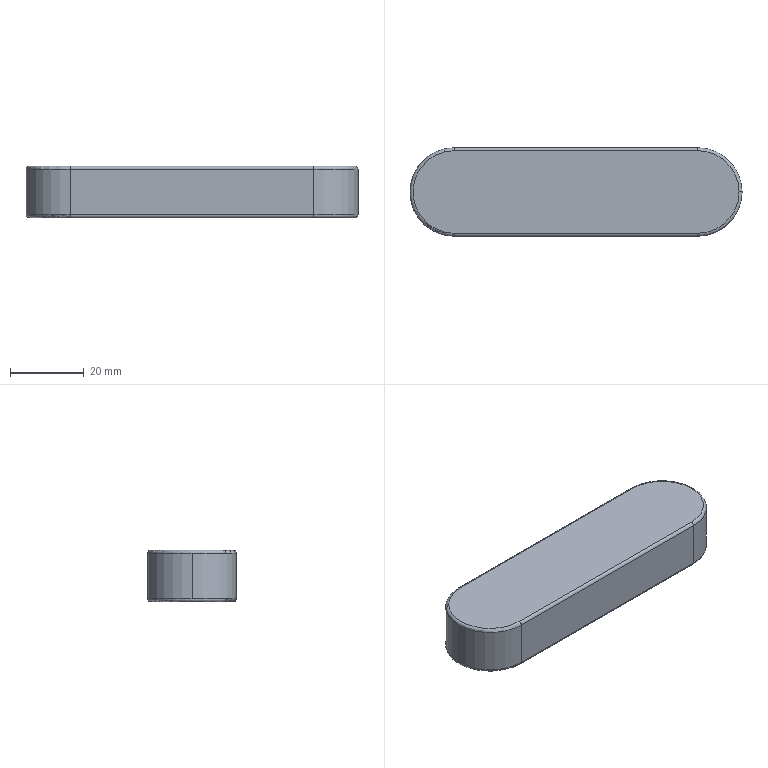Part | STEP file | GB/T1096-1979 plain key, type A, 24×90 | 1 solid | 17 faces | box 90 x 24 x 14 mm | volume 28453 mm3 | cylinder 7 | torus 6 | plane 4 | commonest cylinder face diameters 1.6 x4 24 x3
STEP:
#1=CARTESIAN_POINT('',(0.,0.,0.));
#2=DIRECTION('',(0.,0.,1.));
#3=DIRECTION('',(1.,0.,0.));
#4=AXIS2_PLACEMENT_3D('',#1,#2,#3);
#5=CARTESIAN_POINT('',(44.2,0.,0.));
#6=VERTEX_POINT('',#5);
#7=CARTESIAN_POINT('',(33.,-11.2,0.));
#8=VERTEX_POINT('',#7);
#9=CARTESIAN_POINT('',(33.,0.,0.));
#10=DIRECTION('',(0.,0.,-1.));
#11=DIRECTION('',(1.,0.,0.));
#12=AXIS2_PLACEMENT_3D('',#9,#10,#11);
#13=CIRCLE('',#12,11.2);
#14=CARTESIAN_POINT('',(33.,0.,0.8));
#15=DIRECTION('',(0.,0.,1.));
#16=DIRECTION('',(1.,0.,0.));
#17=AXIS2_PLACEMENT_3D('',#14,#15,#16);
#18=TOROIDAL_SURFACE('',#17,11.2,0.8);
#19=CARTESIAN_POINT('',(6.283,4.712));
#20=DIRECTION('',(-1.,0.));
#21=VECTOR('',#20,1.);
#22=LINE('',#19,#21);
#23=(GEOMETRIC_REPRESENTATION_CONTEXT(2)PARAMETRIC_REPRESENTATION_CONTEXT()REPRESENTATION_CONTEXT('',''));
#24=DEFINITIONAL_REPRESENTATION('',(#22),#23);
#25=PCURVE('',#18,#24);
#26=CARTESIAN_POINT('',(-33.,0.,0.));
#27=DIRECTION('',(0.,0.,1.));
#28=DIRECTION('',(1.,0.,0.));
#29=AXIS2_PLACEMENT_3D('',#26,#27,#28);
#30=PLANE('',#29);
#31=CARTESIAN_POINT('',(77.2,0.));
#32=CARTESIAN_POINT('',(77.2,-19.399));
#33=CARTESIAN_POINT('',(60.4,-9.699));
#34=CARTESIAN_POINT('',(43.6,0.));
#35=CARTESIAN_POINT('',(60.4,9.699));
#36=CARTESIAN_POINT('',(77.2,19.399));
#37=CARTESIAN_POINT('',(77.2,0.));
#38=(BOUNDED_CURVE()B_SPLINE_CURVE(2,(#31,#32,#33,#34,#35,#36,#37),.UNSPECIFIED.,.T.,.F.)B_SPLINE_CURVE_WITH_KNOTS((1,2,2,2,2,1),(-2.094,0.,2.094,4.189,6.283,8.378),.UNSPECIFIED.)CURVE()GEOMETRIC_REPRESENTATION_ITEM()RATIONAL_B_SPLINE_CURVE((1.,0.5,1.,0.5,1.,0.5,1.))REPRESENTATION_ITEM(''));
#39=(GEOMETRIC_REPRESENTATION_CONTEXT(2)PARAMETRIC_REPRESENTATION_CONTEXT()REPRESENTATION_CONTEXT('',''));
#40=DEFINITIONAL_REPRESENTATION('',(#38),#39);
#41=PCURVE('',#30,#40);
#42=SURFACE_CURVE('',#13,(#25,#41),.PCURVE_S1.);
#43=EDGE_CURVE('',#6,#8,#42,.T.);
#44=ORIENTED_EDGE('',*,*,#43,.F.);
#45=CARTESIAN_POINT('',(45.,0.,0.8));
#46=VERTEX_POINT('',#45);
#47=CARTESIAN_POINT('',(44.2,0.,0.8));
#48=DIRECTION('',(0.,-1.,0.));
#49=DIRECTION('',(0.,0.,-1.));
#50=AXIS2_PLACEMENT_3D('',#47,#48,#49);
#51=CIRCLE('',#50,0.8);
#52=CARTESIAN_POINT('',(6.283,4.712));
#53=DIRECTION('',(0.,1.));
#54=VECTOR('',#53,1.);
#55=LINE('',#52,#54);
#56=(GEOMETRIC_REPRESENTATION_CONTEXT(2)PARAMETRIC_REPRESENTATION_CONTEXT()REPRESENTATION_CONTEXT('',''));
#57=DEFINITIONAL_REPRESENTATION('',(#55),#56);
#58=PCURVE('',#18,#57);
#59=CARTESIAN_POINT('',(33.,0.,0.8));
#60=DIRECTION('',(0.,0.,1.));
#61=DIRECTION('',(1.,0.,0.));
#62=AXIS2_PLACEMENT_3D('',#59,#60,#61);
#63=TOROIDAL_SURFACE('',#62,11.2,0.8);
#64=CARTESIAN_POINT('',(0.,4.712));
#65=DIRECTION('',(0.,1.));
#66=VECTOR('',#65,1.);
#67=LINE('',#64,#66);
#68=(GEOMETRIC_REPRESENTATION_CONTEXT(2)PARAMETRIC_REPRESENTATION_CONTEXT()REPRESENTATION_CONTEXT('',''));
#69=DEFINITIONAL_REPRESENTATION('',(#67),#68);
#70=PCURVE('',#63,#69);
#71=SURFACE_CURVE('',#51,(#58,#70),.PCURVE_S1.);
#72=EDGE_CURVE('',#6,#46,#71,.T.);
#73=ORIENTED_EDGE('',*,*,#72,.T.);
#74=CARTESIAN_POINT('',(33.,-12.,0.8));
#75=VERTEX_POINT('',#74);
#76=CARTESIAN_POINT('',(33.,0.,0.8));
#77=DIRECTION('',(0.,0.,1.));
#78=DIRECTION('',(1.,0.,0.));
#79=AXIS2_PLACEMENT_3D('',#76,#77,#78);
#80=CIRCLE('',#79,12.);
#81=CARTESIAN_POINT('',(0.,6.283));
#82=DIRECTION('',(1.,0.));
#83=VECTOR('',#82,1.);
#84=LINE('',#81,#83);
#85=(GEOMETRIC_REPRESENTATION_CONTEXT(2)PARAMETRIC_REPRESENTATION_CONTEXT()REPRESENTATION_CONTEXT('',''));
#86=DEFINITIONAL_REPRESENTATION('',(#84),#85);
#87=PCURVE('',#18,#86);
#88=CARTESIAN_POINT('',(33.,0.,14.));
#89=DIRECTION('',(0.,0.,-1.));
#90=DIRECTION('',(-1.,0.,0.));
#91=AXIS2_PLACEMENT_3D('',#88,#89,#90);
#92=CYLINDRICAL_SURFACE('',#91,12.);
#93=CARTESIAN_POINT('',(9.425,13.2));
#94=DIRECTION('',(-1.,0.));
#95=VECTOR('',#94,1.);
#96=LINE('',#93,#95);
#97=(GEOMETRIC_REPRESENTATION_CONTEXT(2)PARAMETRIC_REPRESENTATION_CONTEXT()REPRESENTATION_CONTEXT('',''));
#98=DEFINITIONAL_REPRESENTATION('',(#96),#97);
#99=PCURVE('',#92,#98);
#100=SURFACE_CURVE('',#80,(#87,#99),.PCURVE_S1.);
#101=EDGE_CURVE('',#75,#46,#100,.T.);
#102=ORIENTED_EDGE('',*,*,#101,.F.);
#103=CARTESIAN_POINT('',(33.,-11.2,0.8));
#104=DIRECTION('',(1.,0.,0.));
#105=DIRECTION('',(0.,0.,-1.));
#106=AXIS2_PLACEMENT_3D('',#103,#104,#105);
#107=CIRCLE('',#106,0.8);
#108=CARTESIAN_POINT('',(4.712,10.996));
#109=DIRECTION('',(0.,-1.));
#110=VECTOR('',#109,1.);
#111=LINE('',#108,#110);
#112=(GEOMETRIC_REPRESENTATION_CONTEXT(2)PARAMETRIC_REPRESENTATION_CONTEXT()REPRESENTATION_CONTEXT('',''));
#113=DEFINITIONAL_REPRESENTATION('',(#111),#112);
#114=PCURVE('',#18,#113);
#115=CARTESIAN_POINT('',(-33.,-11.2,0.8));
#116=DIRECTION('',(1.,0.,0.));
#117=DIRECTION('',(0.,1.,0.));
#118=AXIS2_PLACEMENT_3D('',#115,#116,#117);
#119=CYLINDRICAL_SURFACE('',#118,0.8);
#120=CARTESIAN_POINT('',(-1.571,66.));
#121=DIRECTION('',(1.,0.));
#122=VECTOR('',#121,1.);
#123=LINE('',#120,#122);
#124=(GEOMETRIC_REPRESENTATION_CONTEXT(2)PARAMETRIC_REPRESENTATION_CONTEXT()REPRESENTATION_CONTEXT('',''));
#125=DEFINITIONAL_REPRESENTATION('',(#123),#124);
#126=PCURVE('',#119,#125);
#127=SURFACE_CURVE('',#107,(#114,#126),.PCURVE_S1.);
#128=EDGE_CURVE('',#75,#8,#127,.T.);
#129=ORIENTED_EDGE('',*,*,#128,.T.);
#130=EDGE_LOOP('',(#44,#73,#102,#129));
#131=FACE_BOUND('',#130,.T.);
#132=ADVANCED_FACE('',(#131),#18,.T.);
#133=CARTESIAN_POINT('',(45.,0.,13.2));
#134=VERTEX_POINT('',#133);
#135=CARTESIAN_POINT('',(33.,-12.,13.2));
#136=VERTEX_POINT('',#135);
#137=CARTESIAN_POINT('',(33.,0.,13.2));
#138=DIRECTION('',(0.,0.,-1.));
#139=DIRECTION('',(1.,0.,0.));
#140=AXIS2_PLACEMENT_3D('',#137,#138,#139);
#141=CIRCLE('',#140,12.);
#142=CARTESIAN_POINT('',(33.,0.,13.2));
#143=DIRECTION('',(0.,0.,1.));
#144=DIRECTION('',(1.,0.,0.));
#145=AXIS2_PLACEMENT_3D('',#142,#143,#144);
#146=TOROIDAL_SURFACE('',#145,11.2,0.8);
#147=CARTESIAN_POINT('',(6.283,0.));
#148=DIRECTION('',(-1.,0.));
#149=VECTOR('',#148,1.);
#150=LINE('',#147,#149);
#151=(GEOMETRIC_REPRESENTATION_CONTEXT(2)PARAMETRIC_REPRESENTATION_CONTEXT()REPRESENTATION_CONTEXT('',''));
#152=DEFINITIONAL_REPRESENTATION('',(#150),#151);
#153=PCURVE('',#146,#152);
#154=CARTESIAN_POINT('',(3.142,0.8));
#155=DIRECTION('',(1.,0.));
#156=VECTOR('',#155,1.);
#157=LINE('',#154,#156);
#158=(GEOMETRIC_REPRESENTATION_CONTEXT(2)PARAMETRIC_REPRESENTATION_CONTEXT()REPRESENTATION_CONTEXT('',''));
#159=DEFINITIONAL_REPRESENTATION('',(#157),#158);
#160=PCURVE('',#92,#159);
#161=SURFACE_CURVE('',#141,(#153,#160),.PCURVE_S1.);
#162=EDGE_CURVE('',#134,#136,#161,.T.);
#163=ORIENTED_EDGE('',*,*,#162,.F.);
#164=CARTESIAN_POINT('',(44.2,0.,14.));
#165=VERTEX_POINT('',#164);
#166=CARTESIAN_POINT('',(44.2,0.,13.2));
#167=DIRECTION('',(0.,-1.,0.));
#168=DIRECTION('',(0.,0.,-1.));
#169=AXIS2_PLACEMENT_3D('',#166,#167,#168);
#170=CIRCLE('',#169,0.8);
#171=CARTESIAN_POINT('',(6.283,-1.571));
#172=DIRECTION('',(0.,1.));
#173=VECTOR('',#172,1.);
#174=LINE('',#171,#173);
#175=(GEOMETRIC_REPRESENTATION_CONTEXT(2)PARAMETRIC_REPRESENTATION_CONTEXT()REPRESENTATION_CONTEXT('',''));
#176=DEFINITIONAL_REPRESENTATION('',(#174),#175);
#177=PCURVE('',#146,#176);
#178=CARTESIAN_POINT('',(33.,0.,13.2));
#179=DIRECTION('',(0.,0.,1.));
#180=DIRECTION('',(1.,0.,0.));
#181=AXIS2_PLACEMENT_3D('',#178,#179,#180);
#182=TOROIDAL_SURFACE('',#181,11.2,0.8);
#183=CARTESIAN_POINT('',(0.,-1.571));
#184=DIRECTION('',(0.,1.));
#185=VECTOR('',#184,1.);
#186=LINE('',#183,#185);
#187=(GEOMETRIC_REPRESENTATION_CONTEXT(2)PARAMETRIC_REPRESENTATION_CONTEXT()REPRESENTATION_CONTEXT('',''));
#188=DEFINITIONAL_REPRESENTATION('',(#186),#187);
#189=PCURVE('',#182,#188);
#190=SURFACE_CURVE('',#170,(#177,#189),.PCURVE_S1.);
#191=EDGE_CURVE('',#134,#165,#190,.T.);
#192=ORIENTED_EDGE('',*,*,#191,.T.);
#193=CARTESIAN_POINT('',(33.,-11.2,14.));
#194=VERTEX_POINT('',#193);
#195=CARTESIAN_POINT('',(33.,0.,14.));
#196=DIRECTION('',(0.,0.,1.));
#197=DIRECTION('',(1.,0.,0.));
#198=AXIS2_PLACEMENT_3D('',#195,#196,#197);
#199=CIRCLE('',#198,11.2);
#200=CARTESIAN_POINT('',(0.,1.571));
#201=DIRECTION('',(1.,0.));
#202=VECTOR('',#201,1.);
#203=LINE('',#200,#202);
#204=(GEOMETRIC_REPRESENTATION_CONTEXT(2)PARAMETRIC_REPRESENTATION_CONTEXT()REPRESENTATION_CONTEXT('',''));
#205=DEFINITIONAL_REPRESENTATION('',(#203),#204);
#206=PCURVE('',#146,#205);
#207=CARTESIAN_POINT('',(-33.,0.,14.));
#208=DIRECTION('',(0.,0.,1.));
#209=DIRECTION('',(1.,0.,0.));
#210=AXIS2_PLACEMENT_3D('',#207,#208,#209);
#211=PLANE('',#210);
#212=CARTESIAN_POINT('',(66.,0.));
#213=DIRECTION('',(1.,0.));
#214=AXIS2_PLACEMENT_2D('',#212,#213);
#215=CIRCLE('',#214,11.2);
#216=(GEOMETRIC_REPRESENTATION_CONTEXT(2)PARAMETRIC_REPRESENTATION_CONTEXT()REPRESENTATION_CONTEXT('',''));
#217=DEFINITIONAL_REPRESENTATION('',(#215),#216);
#218=PCURVE('',#211,#217);
#219=SURFACE_CURVE('',#199,(#206,#218),.PCURVE_S1.);
#220=EDGE_CURVE('',#194,#165,#219,.T.);
#221=ORIENTED_EDGE('',*,*,#220,.F.);
#222=CARTESIAN_POINT('',(33.,-11.2,13.2));
#223=DIRECTION('',(1.,0.,0.));
#224=DIRECTION('',(0.,0.,-1.));
#225=AXIS2_PLACEMENT_3D('',#222,#223,#224);
#226=CIRCLE('',#225,0.8);
#227=CARTESIAN_POINT('',(4.712,4.712));
#228=DIRECTION('',(0.,-1.));
#229=VECTOR('',#228,1.);
#230=LINE('',#227,#229);
#231=(GEOMETRIC_REPRESENTATION_CONTEXT(2)PARAMETRIC_REPRESENTATION_CONTEXT()REPRESENTATION_CONTEXT('',''));
#232=DEFINITIONAL_REPRESENTATION('',(#230),#231);
#233=PCURVE('',#146,#232);
#234=CARTESIAN_POINT('',(-33.,-11.2,13.2));
#235=DIRECTION('',(-1.,0.,0.));
#236=DIRECTION('',(0.,-1.,0.));
#237=AXIS2_PLACEMENT_3D('',#234,#235,#236);
#238=CYLINDRICAL_SURFACE('',#237,0.8);
#239=CARTESIAN_POINT('',(4.712,-66.));
#240=DIRECTION('',(-1.,0.));
#241=VECTOR('',#240,1.);
#242=LINE('',#239,#241);
#243=(GEOMETRIC_REPRESENTATION_CONTEXT(2)PARAMETRIC_REPRESENTATION_CONTEXT()REPRESENTATION_CONTEXT('',''));
#244=DEFINITIONAL_REPRESENTATION('',(#242),#243);
#245=PCURVE('',#238,#244);
#246=SURFACE_CURVE('',#226,(#233,#245),.PCURVE_S1.);
#247=EDGE_CURVE('',#194,#136,#246,.T.);
#248=ORIENTED_EDGE('',*,*,#247,.T.);
#249=EDGE_LOOP('',(#163,#192,#221,#248));
#250=FACE_BOUND('',#249,.T.);
#251=ADVANCED_FACE('',(#250),#146,.T.);
#252=CARTESIAN_POINT('',(-33.,-12.,13.2));
#253=VERTEX_POINT('',#252);
#254=CARTESIAN_POINT('',(-45.,0.,13.2));
#255=VERTEX_POINT('',#254);
#256=CARTESIAN_POINT('',(-33.,0.,13.2));
#257=DIRECTION('',(0.,0.,-1.));
#258=DIRECTION('',(1.,0.,0.));
#259=AXIS2_PLACEMENT_3D('',#256,#257,#258);
#260=CIRCLE('',#259,12.);
#261=CARTESIAN_POINT('',(-33.,0.,14.));
#262=DIRECTION('',(0.,0.,-1.));
#263=DIRECTION('',(-1.,0.,0.));
#264=AXIS2_PLACEMENT_3D('',#261,#262,#263);
#265=CYLINDRICAL_SURFACE('',#264,12.);
#266=CARTESIAN_POINT('',(3.142,0.8));
#267=DIRECTION('',(1.,0.));
#268=VECTOR('',#267,1.);
#269=LINE('',#266,#268);
#270=(GEOMETRIC_REPRESENTATION_CONTEXT(2)PARAMETRIC_REPRESENTATION_CONTEXT()REPRESENTATION_CONTEXT('',''));
#271=DEFINITIONAL_REPRESENTATION('',(#269),#270);
#272=PCURVE('',#265,#271);
#273=CARTESIAN_POINT('',(-33.,0.,13.2));
#274=DIRECTION('',(0.,0.,1.));
#275=DIRECTION('',(1.,0.,0.));
#276=AXIS2_PLACEMENT_3D('',#273,#274,#275);
#277=TOROIDAL_SURFACE('',#276,11.2,0.8);
#278=CARTESIAN_POINT('',(6.283,0.));
#279=DIRECTION('',(-1.,0.));
#280=VECTOR('',#279,1.);
#281=LINE('',#278,#280);
#282=(GEOMETRIC_REPRESENTATION_CONTEXT(2)PARAMETRIC_REPRESENTATION_CONTEXT()REPRESENTATION_CONTEXT('',''));
#283=DEFINITIONAL_REPRESENTATION('',(#281),#282);
#284=PCURVE('',#277,#283);
#285=SURFACE_CURVE('',#260,(#272,#284),.PCURVE_S1.);
#286=EDGE_CURVE('',#253,#255,#285,.T.);
#287=ORIENTED_EDGE('',*,*,#286,.T.);
#288=CARTESIAN_POINT('',(-45.,0.,0.8));
#289=VERTEX_POINT('',#288);
#290=CARTESIAN_POINT('',(-45.,0.,14.));
#291=DIRECTION('',(0.,0.,-1.));
#292=VECTOR('',#291,1.);
#293=LINE('',#290,#292);
#294=CARTESIAN_POINT('',(6.283,0.));
#295=DIRECTION('',(0.,1.));
#296=VECTOR('',#295,1.);
#297=LINE('',#294,#296);
#298=(GEOMETRIC_REPRESENTATION_CONTEXT(2)PARAMETRIC_REPRESENTATION_CONTEXT()REPRESENTATION_CONTEXT('',''));
#299=DEFINITIONAL_REPRESENTATION('',(#297),#298);
#300=PCURVE('',#265,#299);
#301=CARTESIAN_POINT('',(-33.,0.,14.));
#302=DIRECTION('',(0.,0.,-1.));
#303=DIRECTION('',(-1.,0.,0.));
#304=AXIS2_PLACEMENT_3D('',#301,#302,#303);
#305=CYLINDRICAL_SURFACE('',#304,12.);
#306=CARTESIAN_POINT('',(0.,0.));
#307=DIRECTION('',(0.,1.));
#308=VECTOR('',#307,1.);
#309=LINE('',#306,#308);
#310=(GEOMETRIC_REPRESENTATION_CONTEXT(2)PARAMETRIC_REPRESENTATION_CONTEXT()REPRESENTATION_CONTEXT('',''));
#311=DEFINITIONAL_REPRESENTATION('',(#309),#310);
#312=PCURVE('',#305,#311);
#313=SURFACE_CURVE('',#293,(#300,#312),.PCURVE_S1.);
#314=EDGE_CURVE('',#255,#289,#313,.T.);
#315=ORIENTED_EDGE('',*,*,#314,.T.);
#316=CARTESIAN_POINT('',(-33.,-12.,0.8));
#317=VERTEX_POINT('',#316);
#318=CARTESIAN_POINT('',(-33.,0.,0.8));
#319=DIRECTION('',(0.,0.,1.));
#320=DIRECTION('',(1.,0.,0.));
#321=AXIS2_PLACEMENT_3D('',#318,#319,#320);
#322=CIRCLE('',#321,12.);
#323=CARTESIAN_POINT('',(9.425,13.2));
#324=DIRECTION('',(-1.,0.));
#325=VECTOR('',#324,1.);
#326=LINE('',#323,#325);
#327=(GEOMETRIC_REPRESENTATION_CONTEXT(2)PARAMETRIC_REPRESENTATION_CONTEXT()REPRESENTATION_CONTEXT('',''));
#328=DEFINITIONAL_REPRESENTATION('',(#326),#327);
#329=PCURVE('',#265,#328);
#330=CARTESIAN_POINT('',(-33.,0.,0.8));
#331=DIRECTION('',(0.,0.,1.));
#332=DIRECTION('',(1.,0.,0.));
#333=AXIS2_PLACEMENT_3D('',#330,#331,#332);
#334=TOROIDAL_SURFACE('',#333,11.2,0.8);
#335=CARTESIAN_POINT('',(0.,6.283));
#336=DIRECTION('',(1.,0.));
#337=VECTOR('',#336,1.);
#338=LINE('',#335,#337);
#339=(GEOMETRIC_REPRESENTATION_CONTEXT(2)PARAMETRIC_REPRESENTATION_CONTEXT()REPRESENTATION_CONTEXT('',''));
#340=DEFINITIONAL_REPRESENTATION('',(#338),#339);
#341=PCURVE('',#334,#340);
#342=SURFACE_CURVE('',#322,(#329,#341),.PCURVE_S1.);
#343=EDGE_CURVE('',#289,#317,#342,.T.);
#344=ORIENTED_EDGE('',*,*,#343,.T.);
#345=CARTESIAN_POINT('',(-33.,-12.,14.));
#346=DIRECTION('',(0.,0.,-1.));
#347=VECTOR('',#346,1.);
#348=LINE('',#345,#347);
#349=CARTESIAN_POINT('',(4.712,0.));
#350=DIRECTION('',(0.,1.));
#351=VECTOR('',#350,1.);
#352=LINE('',#349,#351);
#353=(GEOMETRIC_REPRESENTATION_CONTEXT(2)PARAMETRIC_REPRESENTATION_CONTEXT()REPRESENTATION_CONTEXT('',''));
#354=DEFINITIONAL_REPRESENTATION('',(#352),#353);
#355=PCURVE('',#265,#354);
#356=CARTESIAN_POINT('',(-33.,-12.,14.));
#357=DIRECTION('',(0.,1.,0.));
#358=DIRECTION('',(-1.,0.,0.));
#359=AXIS2_PLACEMENT_3D('',#356,#357,#358);
#360=PLANE('',#359);
#361=CARTESIAN_POINT('',(0.,0.));
#362=DIRECTION('',(0.,-1.));
#363=VECTOR('',#362,1.);
#364=LINE('',#361,#363);
#365=(GEOMETRIC_REPRESENTATION_CONTEXT(2)PARAMETRIC_REPRESENTATION_CONTEXT()REPRESENTATION_CONTEXT('',''));
#366=DEFINITIONAL_REPRESENTATION('',(#364),#365);
#367=PCURVE('',#360,#366);
#368=SURFACE_CURVE('',#348,(#355,#367),.PCURVE_S1.);
#369=EDGE_CURVE('',#253,#317,#368,.T.);
#370=ORIENTED_EDGE('',*,*,#369,.F.);
#371=EDGE_LOOP('',(#287,#315,#344,#370));
#372=FACE_BOUND('',#371,.T.);
#373=ADVANCED_FACE('',(#372),#265,.T.);
#374=ORIENTED_EDGE('',*,*,#314,.F.);
#375=CARTESIAN_POINT('',(-33.,12.,13.2));
#376=VERTEX_POINT('',#375);
#377=CARTESIAN_POINT('',(-33.,0.,13.2));
#378=DIRECTION('',(0.,0.,-1.));
#379=DIRECTION('',(1.,0.,0.));
#380=AXIS2_PLACEMENT_3D('',#377,#378,#379);
#381=CIRCLE('',#380,12.);
#382=CARTESIAN_POINT('',(-3.142,0.8));
#383=DIRECTION('',(1.,0.));
#384=VECTOR('',#383,1.);
#385=LINE('',#382,#384);
#386=(GEOMETRIC_REPRESENTATION_CONTEXT(2)PARAMETRIC_REPRESENTATION_CONTEXT()REPRESENTATION_CONTEXT('',''));
#387=DEFINITIONAL_REPRESENTATION('',(#385),#386);
#388=PCURVE('',#305,#387);
#389=CARTESIAN_POINT('',(6.283,0.));
#390=DIRECTION('',(-1.,0.));
#391=VECTOR('',#390,1.);
#392=LINE('',#389,#391);
#393=(GEOMETRIC_REPRESENTATION_CONTEXT(2)PARAMETRIC_REPRESENTATION_CONTEXT()REPRESENTATION_CONTEXT('',''));
#394=DEFINITIONAL_REPRESENTATION('',(#392),#393);
#395=PCURVE('',#277,#394);
#396=SURFACE_CURVE('',#381,(#388,#395),.PCURVE_S1.);
#397=EDGE_CURVE('',#255,#376,#396,.T.);
#398=ORIENTED_EDGE('',*,*,#397,.T.);
#399=CARTESIAN_POINT('',(-33.,12.,0.8));
#400=VERTEX_POINT('',#399);
#401=CARTESIAN_POINT('',(-33.,12.,14.));
#402=DIRECTION('',(0.,0.,-1.));
#403=VECTOR('',#402,1.);
#404=LINE('',#401,#403);
#405=CARTESIAN_POINT('',(1.571,0.));
#406=DIRECTION('',(0.,1.));
#407=VECTOR('',#406,1.);
#408=LINE('',#405,#407);
#409=(GEOMETRIC_REPRESENTATION_CONTEXT(2)PARAMETRIC_REPRESENTATION_CONTEXT()REPRESENTATION_CONTEXT('',''));
#410=DEFINITIONAL_REPRESENTATION('',(#408),#409);
#411=PCURVE('',#305,#410);
#412=CARTESIAN_POINT('',(-33.,12.,14.));
#413=DIRECTION('',(0.,-1.,0.));
#414=DIRECTION('',(1.,0.,0.));
#415=AXIS2_PLACEMENT_3D('',#412,#413,#414);
#416=PLANE('',#415);
#417=CARTESIAN_POINT('',(0.,0.));
#418=DIRECTION('',(0.,-1.));
#419=VECTOR('',#418,1.);
#420=LINE('',#417,#419);
#421=(GEOMETRIC_REPRESENTATION_CONTEXT(2)PARAMETRIC_REPRESENTATION_CONTEXT()REPRESENTATION_CONTEXT('',''));
#422=DEFINITIONAL_REPRESENTATION('',(#420),#421);
#423=PCURVE('',#416,#422);
#424=SURFACE_CURVE('',#404,(#411,#423),.PCURVE_S1.);
#425=EDGE_CURVE('',#376,#400,#424,.T.);
#426=ORIENTED_EDGE('',*,*,#425,.T.);
#427=CARTESIAN_POINT('',(-33.,0.,0.8));
#428=DIRECTION('',(0.,0.,1.));
#429=DIRECTION('',(1.,0.,0.));
#430=AXIS2_PLACEMENT_3D('',#427,#428,#429);
#431=CIRCLE('',#430,12.);
#432=CARTESIAN_POINT('',(3.142,13.2));
#433=DIRECTION('',(-1.,0.));
#434=VECTOR('',#433,1.);
#435=LINE('',#432,#434);
#436=(GEOMETRIC_REPRESENTATION_CONTEXT(2)PARAMETRIC_REPRESENTATION_CONTEXT()REPRESENTATION_CONTEXT('',''));
#437=DEFINITIONAL_REPRESENTATION('',(#435),#436);
#438=PCURVE('',#305,#437);
#439=CARTESIAN_POINT('',(0.,6.283));
#440=DIRECTION('',(1.,0.));
#441=VECTOR('',#440,1.);
#442=LINE('',#439,#441);
#443=(GEOMETRIC_REPRESENTATION_CONTEXT(2)PARAMETRIC_REPRESENTATION_CONTEXT()REPRESENTATION_CONTEXT('',''));
#444=DEFINITIONAL_REPRESENTATION('',(#442),#443);
#445=PCURVE('',#334,#444);
#446=SURFACE_CURVE('',#431,(#438,#445),.PCURVE_S1.);
#447=EDGE_CURVE('',#400,#289,#446,.T.);
#448=ORIENTED_EDGE('',*,*,#447,.T.);
#449=EDGE_LOOP('',(#374,#398,#426,#448));
#450=FACE_BOUND('',#449,.T.);
#451=ADVANCED_FACE('',(#450),#305,.T.);
#452=CARTESIAN_POINT('',(33.,-12.,14.));
#453=DIRECTION('',(0.,0.,-1.));
#454=VECTOR('',#453,1.);
#455=LINE('',#452,#454);
#456=CARTESIAN_POINT('',(-66.,0.));
#457=DIRECTION('',(0.,-1.));
#458=VECTOR('',#457,1.);
#459=LINE('',#456,#458);
#460=(GEOMETRIC_REPRESENTATION_CONTEXT(2)PARAMETRIC_REPRESENTATION_CONTEXT()REPRESENTATION_CONTEXT('',''));
#461=DEFINITIONAL_REPRESENTATION('',(#459),#460);
#462=PCURVE('',#360,#461);
#463=CARTESIAN_POINT('',(4.712,0.));
#464=DIRECTION('',(0.,1.));
#465=VECTOR('',#464,1.);
#466=LINE('',#463,#465);
#467=(GEOMETRIC_REPRESENTATION_CONTEXT(2)PARAMETRIC_REPRESENTATION_CONTEXT()REPRESENTATION_CONTEXT('',''));
#468=DEFINITIONAL_REPRESENTATION('',(#466),#467);
#469=PCURVE('',#92,#468);
#470=SURFACE_CURVE('',#455,(#462,#469),.PCURVE_S1.);
#471=EDGE_CURVE('',#136,#75,#470,.T.);
#472=ORIENTED_EDGE('',*,*,#471,.F.);
#473=CARTESIAN_POINT('',(-33.,-12.,13.2));
#474=DIRECTION('',(-1.,0.,0.));
#475=VECTOR('',#474,1.);
#476=LINE('',#473,#475);
#477=CARTESIAN_POINT('',(0.,-0.8));
#478=DIRECTION('',(1.,0.));
#479=VECTOR('',#478,1.);
#480=LINE('',#477,#479);
#481=(GEOMETRIC_REPRESENTATION_CONTEXT(2)PARAMETRIC_REPRESENTATION_CONTEXT()REPRESENTATION_CONTEXT('',''));
#482=DEFINITIONAL_REPRESENTATION('',(#480),#481);
#483=PCURVE('',#360,#482);
#484=CARTESIAN_POINT('',(0.,0.));
#485=DIRECTION('',(0.,1.));
#486=VECTOR('',#485,1.);
#487=LINE('',#484,#486);
#488=(GEOMETRIC_REPRESENTATION_CONTEXT(2)PARAMETRIC_REPRESENTATION_CONTEXT()REPRESENTATION_CONTEXT('',''));
#489=DEFINITIONAL_REPRESENTATION('',(#487),#488);
#490=PCURVE('',#238,#489);
#491=SURFACE_CURVE('',#476,(#483,#490),.PCURVE_S1.);
#492=EDGE_CURVE('',#136,#253,#491,.T.);
#493=ORIENTED_EDGE('',*,*,#492,.T.);
#494=ORIENTED_EDGE('',*,*,#369,.T.);
#495=CARTESIAN_POINT('',(-33.,-12.,0.8));
#496=DIRECTION('',(1.,0.,0.));
#497=VECTOR('',#496,1.);
#498=LINE('',#495,#497);
#499=CARTESIAN_POINT('',(0.,-13.2));
#500=DIRECTION('',(-1.,0.));
#501=VECTOR('',#500,1.);
#502=LINE('',#499,#501);
#503=(GEOMETRIC_REPRESENTATION_CONTEXT(2)PARAMETRIC_REPRESENTATION_CONTEXT()REPRESENTATION_CONTEXT('',''));
#504=DEFINITIONAL_REPRESENTATION('',(#502),#503);
#505=PCURVE('',#360,#504);
#506=CARTESIAN_POINT('',(3.142,0.));
#507=DIRECTION('',(0.,1.));
#508=VECTOR('',#507,1.);
#509=LINE('',#506,#508);
#510=(GEOMETRIC_REPRESENTATION_CONTEXT(2)PARAMETRIC_REPRESENTATION_CONTEXT()REPRESENTATION_CONTEXT('',''));
#511=DEFINITIONAL_REPRESENTATION('',(#509),#510);
#512=PCURVE('',#119,#511);
#513=SURFACE_CURVE('',#498,(#505,#512),.PCURVE_S1.);
#514=EDGE_CURVE('',#317,#75,#513,.T.);
#515=ORIENTED_EDGE('',*,*,#514,.T.);
#516=EDGE_LOOP('',(#472,#493,#494,#515));
#517=FACE_BOUND('',#516,.T.);
#518=ADVANCED_FACE('',(#517),#360,.F.);
#519=CARTESIAN_POINT('',(33.,12.,13.2));
#520=VERTEX_POINT('',#519);
#521=CARTESIAN_POINT('',(33.,12.,0.8));
#522=VERTEX_POINT('',#521);
#523=CARTESIAN_POINT('',(33.,12.,14.));
#524=DIRECTION('',(0.,0.,-1.));
#525=VECTOR('',#524,1.);
#526=LINE('',#523,#525);
#527=CARTESIAN_POINT('',(1.571,0.));
#528=DIRECTION('',(0.,1.));
#529=VECTOR('',#528,1.);
#530=LINE('',#527,#529);
#531=(GEOMETRIC_REPRESENTATION_CONTEXT(2)PARAMETRIC_REPRESENTATION_CONTEXT()REPRESENTATION_CONTEXT('',''));
#532=DEFINITIONAL_REPRESENTATION('',(#530),#531);
#533=PCURVE('',#92,#532);
#534=CARTESIAN_POINT('',(66.,0.));
#535=DIRECTION('',(0.,-1.));
#536=VECTOR('',#535,1.);
#537=LINE('',#534,#536);
#538=(GEOMETRIC_REPRESENTATION_CONTEXT(2)PARAMETRIC_REPRESENTATION_CONTEXT()REPRESENTATION_CONTEXT('',''));
#539=DEFINITIONAL_REPRESENTATION('',(#537),#538);
#540=PCURVE('',#416,#539);
#541=SURFACE_CURVE('',#526,(#533,#540),.PCURVE_S1.);
#542=EDGE_CURVE('',#520,#522,#541,.T.);
#543=ORIENTED_EDGE('',*,*,#542,.F.);
#544=CARTESIAN_POINT('',(33.,0.,13.2));
#545=DIRECTION('',(0.,0.,-1.));
#546=DIRECTION('',(1.,0.,0.));
#547=AXIS2_PLACEMENT_3D('',#544,#545,#546);
#548=CIRCLE('',#547,12.);
#549=CARTESIAN_POINT('',(-3.142,0.8));
#550=DIRECTION('',(1.,0.));
#551=VECTOR('',#550,1.);
#552=LINE('',#549,#551);
#553=(GEOMETRIC_REPRESENTATION_CONTEXT(2)PARAMETRIC_REPRESENTATION_CONTEXT()REPRESENTATION_CONTEXT('',''));
#554=DEFINITIONAL_REPRESENTATION('',(#552),#553);
#555=PCURVE('',#92,#554);
#556=CARTESIAN_POINT('',(6.283,0.));
#557=DIRECTION('',(-1.,0.));
#558=VECTOR('',#557,1.);
#559=LINE('',#556,#558);
#560=(GEOMETRIC_REPRESENTATION_CONTEXT(2)PARAMETRIC_REPRESENTATION_CONTEXT()REPRESENTATION_CONTEXT('',''));
#561=DEFINITIONAL_REPRESENTATION('',(#559),#560);
#562=PCURVE('',#182,#561);
#563=SURFACE_CURVE('',#548,(#555,#562),.PCURVE_S1.);
#564=EDGE_CURVE('',#520,#134,#563,.T.);
#565=ORIENTED_EDGE('',*,*,#564,.T.);
#566=ORIENTED_EDGE('',*,*,#162,.T.);
#567=ORIENTED_EDGE('',*,*,#471,.T.);
#568=ORIENTED_EDGE('',*,*,#101,.T.);
#569=CARTESIAN_POINT('',(33.,0.,0.8));
#570=DIRECTION('',(0.,0.,1.));
#571=DIRECTION('',(1.,0.,0.));
#572=AXIS2_PLACEMENT_3D('',#569,#570,#571);
#573=CIRCLE('',#572,12.);
#574=CARTESIAN_POINT('',(3.142,13.2));
#575=DIRECTION('',(-1.,0.));
#576=VECTOR('',#575,1.);
#577=LINE('',#574,#576);
#578=(GEOMETRIC_REPRESENTATION_CONTEXT(2)PARAMETRIC_REPRESENTATION_CONTEXT()REPRESENTATION_CONTEXT('',''));
#579=DEFINITIONAL_REPRESENTATION('',(#577),#578);
#580=PCURVE('',#92,#579);
#581=CARTESIAN_POINT('',(0.,6.283));
#582=DIRECTION('',(1.,0.));
#583=VECTOR('',#582,1.);
#584=LINE('',#581,#583);
#585=(GEOMETRIC_REPRESENTATION_CONTEXT(2)PARAMETRIC_REPRESENTATION_CONTEXT()REPRESENTATION_CONTEXT('',''));
#586=DEFINITIONAL_REPRESENTATION('',(#584),#585);
#587=PCURVE('',#63,#586);
#588=SURFACE_CURVE('',#573,(#580,#587),.PCURVE_S1.);
#589=EDGE_CURVE('',#46,#522,#588,.T.);
#590=ORIENTED_EDGE('',*,*,#589,.T.);
#591=EDGE_LOOP('',(#543,#565,#566,#567,#568,#590));
#592=FACE_BOUND('',#591,.T.);
#593=ADVANCED_FACE('',(#592),#92,.T.);
#594=ORIENTED_EDGE('',*,*,#425,.F.);
#595=CARTESIAN_POINT('',(33.,12.,13.2));
#596=DIRECTION('',(1.,0.,0.));
#597=VECTOR('',#596,1.);
#598=LINE('',#595,#597);
#599=CARTESIAN_POINT('',(66.,-0.8));
#600=DIRECTION('',(1.,0.));
#601=VECTOR('',#600,1.);
#602=LINE('',#599,#601);
#603=(GEOMETRIC_REPRESENTATION_CONTEXT(2)PARAMETRIC_REPRESENTATION_CONTEXT()REPRESENTATION_CONTEXT('',''));
#604=DEFINITIONAL_REPRESENTATION('',(#602),#603);
#605=PCURVE('',#416,#604);
#606=CARTESIAN_POINT('',(-33.,11.2,13.2));
#607=DIRECTION('',(1.,0.,0.));
#608=DIRECTION('',(0.,1.,0.));
#609=AXIS2_PLACEMENT_3D('',#606,#607,#608);
#610=CYLINDRICAL_SURFACE('',#609,0.8);
#611=CARTESIAN_POINT('',(0.,66.));
#612=DIRECTION('',(0.,1.));
#613=VECTOR('',#612,1.);
#614=LINE('',#611,#613);
#615=(GEOMETRIC_REPRESENTATION_CONTEXT(2)PARAMETRIC_REPRESENTATION_CONTEXT()REPRESENTATION_CONTEXT('',''));
#616=DEFINITIONAL_REPRESENTATION('',(#614),#615);
#617=PCURVE('',#610,#616);
#618=SURFACE_CURVE('',#598,(#605,#617),.PCURVE_S1.);
#619=EDGE_CURVE('',#376,#520,#618,.T.);
#620=ORIENTED_EDGE('',*,*,#619,.T.);
#621=ORIENTED_EDGE('',*,*,#542,.T.);
#622=CARTESIAN_POINT('',(-33.,12.,0.8));
#623=DIRECTION('',(-1.,0.,0.));
#624=VECTOR('',#623,1.);
#625=LINE('',#622,#624);
#626=CARTESIAN_POINT('',(0.,-13.2));
#627=DIRECTION('',(-1.,0.));
#628=VECTOR('',#627,1.);
#629=LINE('',#626,#628);
#630=(GEOMETRIC_REPRESENTATION_CONTEXT(2)PARAMETRIC_REPRESENTATION_CONTEXT()REPRESENTATION_CONTEXT('',''));
#631=DEFINITIONAL_REPRESENTATION('',(#629),#630);
#632=PCURVE('',#416,#631);
#633=CARTESIAN_POINT('',(-33.,11.2,0.8));
#634=DIRECTION('',(-1.,0.,0.));
#635=DIRECTION('',(0.,-1.,0.));
#636=AXIS2_PLACEMENT_3D('',#633,#634,#635);
#637=CYLINDRICAL_SURFACE('',#636,0.8);
#638=CARTESIAN_POINT('',(3.142,0.));
#639=DIRECTION('',(0.,1.));
#640=VECTOR('',#639,1.);
#641=LINE('',#638,#640);
#642=(GEOMETRIC_REPRESENTATION_CONTEXT(2)PARAMETRIC_REPRESENTATION_CONTEXT()REPRESENTATION_CONTEXT('',''));
#643=DEFINITIONAL_REPRESENTATION('',(#641),#642);
#644=PCURVE('',#637,#643);
#645=SURFACE_CURVE('',#625,(#632,#644),.PCURVE_S1.);
#646=EDGE_CURVE('',#522,#400,#645,.T.);
#647=ORIENTED_EDGE('',*,*,#646,.T.);
#648=EDGE_LOOP('',(#594,#620,#621,#647));
#649=FACE_BOUND('',#648,.T.);
#650=ADVANCED_FACE('',(#649),#416,.F.);
#651=CARTESIAN_POINT('',(-33.,-11.2,14.));
#652=VERTEX_POINT('',#651);
#653=CARTESIAN_POINT('',(33.,-11.2,14.));
#654=DIRECTION('',(1.,0.,0.));
#655=VECTOR('',#654,1.);
#656=LINE('',#653,#655);
#657=CARTESIAN_POINT('',(66.,-11.2));
#658=DIRECTION('',(1.,0.));
#659=VECTOR('',#658,1.);
#660=LINE('',#657,#659);
#661=(GEOMETRIC_REPRESENTATION_CONTEXT(2)PARAMETRIC_REPRESENTATION_CONTEXT()REPRESENTATION_CONTEXT('',''));
#662=DEFINITIONAL_REPRESENTATION('',(#660),#661);
#663=PCURVE('',#211,#662);
#664=CARTESIAN_POINT('',(1.571,-66.));
#665=DIRECTION('',(0.,-1.));
#666=VECTOR('',#665,1.);
#667=LINE('',#664,#666);
#668=(GEOMETRIC_REPRESENTATION_CONTEXT(2)PARAMETRIC_REPRESENTATION_CONTEXT()REPRESENTATION_CONTEXT('',''));
#669=DEFINITIONAL_REPRESENTATION('',(#667),#668);
#670=PCURVE('',#238,#669);
#671=SURFACE_CURVE('',#656,(#663,#670),.PCURVE_S1.);
#672=EDGE_CURVE('',#652,#194,#671,.T.);
#673=ORIENTED_EDGE('',*,*,#672,.T.);
#674=ORIENTED_EDGE('',*,*,#220,.T.);
#675=CARTESIAN_POINT('',(33.,11.2,14.));
#676=VERTEX_POINT('',#675);
#677=CARTESIAN_POINT('',(33.,0.,14.));
#678=DIRECTION('',(0.,0.,1.));
#679=DIRECTION('',(1.,0.,0.));
#680=AXIS2_PLACEMENT_3D('',#677,#678,#679);
#681=CIRCLE('',#680,11.2);
#682=CARTESIAN_POINT('',(66.,0.));
#683=DIRECTION('',(1.,0.));
#684=AXIS2_PLACEMENT_2D('',#682,#683);
#685=CIRCLE('',#684,11.2);
#686=(GEOMETRIC_REPRESENTATION_CONTEXT(2)PARAMETRIC_REPRESENTATION_CONTEXT()REPRESENTATION_CONTEXT('',''));
#687=DEFINITIONAL_REPRESENTATION('',(#685),#686);
#688=PCURVE('',#211,#687);
#689=CARTESIAN_POINT('',(0.,1.571));
#690=DIRECTION('',(1.,0.));
#691=VECTOR('',#690,1.);
#692=LINE('',#689,#691);
#693=(GEOMETRIC_REPRESENTATION_CONTEXT(2)PARAMETRIC_REPRESENTATION_CONTEXT()REPRESENTATION_CONTEXT('',''));
#694=DEFINITIONAL_REPRESENTATION('',(#692),#693);
#695=PCURVE('',#182,#694);
#696=SURFACE_CURVE('',#681,(#688,#695),.PCURVE_S1.);
#697=EDGE_CURVE('',#165,#676,#696,.T.);
#698=ORIENTED_EDGE('',*,*,#697,.T.);
#699=CARTESIAN_POINT('',(-33.,11.2,14.));
#700=VERTEX_POINT('',#699);
#701=CARTESIAN_POINT('',(-33.,11.2,14.));
#702=DIRECTION('',(-1.,0.,0.));
#703=VECTOR('',#702,1.);
#704=LINE('',#701,#703);
#705=CARTESIAN_POINT('',(0.,11.2));
#706=DIRECTION('',(-1.,0.));
#707=VECTOR('',#706,1.);
#708=LINE('',#705,#707);
#709=(GEOMETRIC_REPRESENTATION_CONTEXT(2)PARAMETRIC_REPRESENTATION_CONTEXT()REPRESENTATION_CONTEXT('',''));
#710=DEFINITIONAL_REPRESENTATION('',(#708),#709);
#711=PCURVE('',#211,#710);
#712=CARTESIAN_POINT('',(1.571,0.));
#713=DIRECTION('',(0.,-1.));
#714=VECTOR('',#713,1.);
#715=LINE('',#712,#714);
#716=(GEOMETRIC_REPRESENTATION_CONTEXT(2)PARAMETRIC_REPRESENTATION_CONTEXT()REPRESENTATION_CONTEXT('',''));
#717=DEFINITIONAL_REPRESENTATION('',(#715),#716);
#718=PCURVE('',#610,#717);
#719=SURFACE_CURVE('',#704,(#711,#718),.PCURVE_S1.);
#720=EDGE_CURVE('',#676,#700,#719,.T.);
#721=ORIENTED_EDGE('',*,*,#720,.T.);
#722=CARTESIAN_POINT('',(-33.,0.,14.));
#723=DIRECTION('',(0.,0.,1.));
#724=DIRECTION('',(1.,0.,0.));
#725=AXIS2_PLACEMENT_3D('',#722,#723,#724);
#726=CIRCLE('',#725,11.2);
#727=CARTESIAN_POINT('',(0.,0.));
#728=DIRECTION('',(1.,0.));
#729=AXIS2_PLACEMENT_2D('',#727,#728);
#730=CIRCLE('',#729,11.2);
#731=(GEOMETRIC_REPRESENTATION_CONTEXT(2)PARAMETRIC_REPRESENTATION_CONTEXT()REPRESENTATION_CONTEXT('',''));
#732=DEFINITIONAL_REPRESENTATION('',(#730),#731);
#733=PCURVE('',#211,#732);
#734=CARTESIAN_POINT('',(0.,1.571));
#735=DIRECTION('',(1.,0.));
#736=VECTOR('',#735,1.);
#737=LINE('',#734,#736);
#738=(GEOMETRIC_REPRESENTATION_CONTEXT(2)PARAMETRIC_REPRESENTATION_CONTEXT()REPRESENTATION_CONTEXT('',''));
#739=DEFINITIONAL_REPRESENTATION('',(#737),#738);
#740=PCURVE('',#277,#739);
#741=SURFACE_CURVE('',#726,(#733,#740),.PCURVE_S1.);
#742=EDGE_CURVE('',#700,#652,#741,.T.);
#743=ORIENTED_EDGE('',*,*,#742,.T.);
#744=EDGE_LOOP('',(#673,#674,#698,#721,#743));
#745=FACE_BOUND('',#744,.T.);
#746=ADVANCED_FACE('',(#745),#211,.T.);
#747=CARTESIAN_POINT('',(-33.,11.2,0.));
#748=VERTEX_POINT('',#747);
#749=CARTESIAN_POINT('',(33.,11.2,0.));
#750=VERTEX_POINT('',#749);
#751=CARTESIAN_POINT('',(-33.,11.2,0.));
#752=DIRECTION('',(1.,0.,0.));
#753=VECTOR('',#752,1.);
#754=LINE('',#751,#753);
#755=CARTESIAN_POINT('',(0.,11.2));
#756=DIRECTION('',(1.,0.));
#757=VECTOR('',#756,1.);
#758=LINE('',#755,#757);
#759=(GEOMETRIC_REPRESENTATION_CONTEXT(2)PARAMETRIC_REPRESENTATION_CONTEXT()REPRESENTATION_CONTEXT('',''));
#760=DEFINITIONAL_REPRESENTATION('',(#758),#759);
#761=PCURVE('',#30,#760);
#762=CARTESIAN_POINT('',(4.712,0.));
#763=DIRECTION('',(0.,-1.));
#764=VECTOR('',#763,1.);
#765=LINE('',#762,#764);
#766=(GEOMETRIC_REPRESENTATION_CONTEXT(2)PARAMETRIC_REPRESENTATION_CONTEXT()REPRESENTATION_CONTEXT('',''));
#767=DEFINITIONAL_REPRESENTATION('',(#765),#766);
#768=PCURVE('',#637,#767);
#769=SURFACE_CURVE('',#754,(#761,#768),.PCURVE_S1.);
#770=EDGE_CURVE('',#748,#750,#769,.T.);
#771=ORIENTED_EDGE('',*,*,#770,.T.);
#772=CARTESIAN_POINT('',(33.,0.,0.));
#773=DIRECTION('',(0.,0.,-1.));
#774=DIRECTION('',(1.,0.,0.));
#775=AXIS2_PLACEMENT_3D('',#772,#773,#774);
#776=CIRCLE('',#775,11.2);
#777=CARTESIAN_POINT('',(77.2,0.));
#778=CARTESIAN_POINT('',(77.2,-19.399));
#779=CARTESIAN_POINT('',(60.4,-9.699));
#780=CARTESIAN_POINT('',(43.6,0.));
#781=CARTESIAN_POINT('',(60.4,9.699));
#782=CARTESIAN_POINT('',(77.2,19.399));
#783=CARTESIAN_POINT('',(77.2,0.));
#784=(BOUNDED_CURVE()B_SPLINE_CURVE(2,(#777,#778,#779,#780,#781,#782,#783),.UNSPECIFIED.,.T.,.F.)B_SPLINE_CURVE_WITH_KNOTS((1,2,2,2,2,1),(-2.094,0.,2.094,4.189,6.283,8.378),.UNSPECIFIED.)CURVE()GEOMETRIC_REPRESENTATION_ITEM()RATIONAL_B_SPLINE_CURVE((1.,0.5,1.,0.5,1.,0.5,1.))REPRESENTATION_ITEM(''));
#785=(GEOMETRIC_REPRESENTATION_CONTEXT(2)PARAMETRIC_REPRESENTATION_CONTEXT()REPRESENTATION_CONTEXT('',''));
#786=DEFINITIONAL_REPRESENTATION('',(#784),#785);
#787=PCURVE('',#30,#786);
#788=CARTESIAN_POINT('',(6.283,4.712));
#789=DIRECTION('',(-1.,0.));
#790=VECTOR('',#789,1.);
#791=LINE('',#788,#790);
#792=(GEOMETRIC_REPRESENTATION_CONTEXT(2)PARAMETRIC_REPRESENTATION_CONTEXT()REPRESENTATION_CONTEXT('',''));
#793=DEFINITIONAL_REPRESENTATION('',(#791),#792);
#794=PCURVE('',#63,#793);
#795=SURFACE_CURVE('',#776,(#787,#794),.PCURVE_S1.);
#796=EDGE_CURVE('',#750,#6,#795,.T.);
#797=ORIENTED_EDGE('',*,*,#796,.T.);
#798=ORIENTED_EDGE('',*,*,#43,.T.);
#799=CARTESIAN_POINT('',(-33.,-11.2,0.));
#800=VERTEX_POINT('',#799);
#801=CARTESIAN_POINT('',(-33.,-11.2,0.));
#802=DIRECTION('',(-1.,0.,0.));
#803=VECTOR('',#802,1.);
#804=LINE('',#801,#803);
#805=CARTESIAN_POINT('',(0.,-11.2));
#806=DIRECTION('',(-1.,0.));
#807=VECTOR('',#806,1.);
#808=LINE('',#805,#807);
#809=(GEOMETRIC_REPRESENTATION_CONTEXT(2)PARAMETRIC_REPRESENTATION_CONTEXT()REPRESENTATION_CONTEXT('',''));
#810=DEFINITIONAL_REPRESENTATION('',(#808),#809);
#811=PCURVE('',#30,#810);
#812=CARTESIAN_POINT('',(4.712,0.));
#813=DIRECTION('',(0.,-1.));
#814=VECTOR('',#813,1.);
#815=LINE('',#812,#814);
#816=(GEOMETRIC_REPRESENTATION_CONTEXT(2)PARAMETRIC_REPRESENTATION_CONTEXT()REPRESENTATION_CONTEXT('',''));
#817=DEFINITIONAL_REPRESENTATION('',(#815),#816);
#818=PCURVE('',#119,#817);
#819=SURFACE_CURVE('',#804,(#811,#818),.PCURVE_S1.);
#820=EDGE_CURVE('',#8,#800,#819,.T.);
#821=ORIENTED_EDGE('',*,*,#820,.T.);
#822=CARTESIAN_POINT('',(-33.,0.,0.));
#823=DIRECTION('',(0.,0.,-1.));
#824=DIRECTION('',(1.,0.,0.));
#825=AXIS2_PLACEMENT_3D('',#822,#823,#824);
#826=CIRCLE('',#825,11.2);
#827=CARTESIAN_POINT('',(11.2,0.));
#828=CARTESIAN_POINT('',(11.2,-19.399));
#829=CARTESIAN_POINT('',(-5.6,-9.699));
#830=CARTESIAN_POINT('',(-22.4,0.));
#831=CARTESIAN_POINT('',(-5.6,9.699));
#832=CARTESIAN_POINT('',(11.2,19.399));
#833=CARTESIAN_POINT('',(11.2,0.));
#834=(BOUNDED_CURVE()B_SPLINE_CURVE(2,(#827,#828,#829,#830,#831,#832,#833),.UNSPECIFIED.,.T.,.F.)B_SPLINE_CURVE_WITH_KNOTS((1,2,2,2,2,1),(-2.094,0.,2.094,4.189,6.283,8.378),.UNSPECIFIED.)CURVE()GEOMETRIC_REPRESENTATION_ITEM()RATIONAL_B_SPLINE_CURVE((1.,0.5,1.,0.5,1.,0.5,1.))REPRESENTATION_ITEM(''));
#835=(GEOMETRIC_REPRESENTATION_CONTEXT(2)PARAMETRIC_REPRESENTATION_CONTEXT()REPRESENTATION_CONTEXT('',''));
#836=DEFINITIONAL_REPRESENTATION('',(#834),#835);
#837=PCURVE('',#30,#836);
#838=CARTESIAN_POINT('',(6.283,4.712));
#839=DIRECTION('',(-1.,0.));
#840=VECTOR('',#839,1.);
#841=LINE('',#838,#840);
#842=(GEOMETRIC_REPRESENTATION_CONTEXT(2)PARAMETRIC_REPRESENTATION_CONTEXT()REPRESENTATION_CONTEXT('',''));
#843=DEFINITIONAL_REPRESENTATION('',(#841),#842);
#844=PCURVE('',#334,#843);
#845=SURFACE_CURVE('',#826,(#837,#844),.PCURVE_S1.);
#846=EDGE_CURVE('',#800,#748,#845,.T.);
#847=ORIENTED_EDGE('',*,*,#846,.T.);
#848=EDGE_LOOP('',(#771,#797,#798,#821,#847));
#849=FACE_BOUND('',#848,.T.);
#850=ADVANCED_FACE('',(#849),#30,.F.);
#851=CARTESIAN_POINT('',(-33.,11.2,13.2));
#852=DIRECTION('',(1.,0.,0.));
#853=DIRECTION('',(0.,0.,-1.));
#854=AXIS2_PLACEMENT_3D('',#851,#852,#853);
#855=CIRCLE('',#854,0.8);
#856=CARTESIAN_POINT('',(1.571,-1.571));
#857=DIRECTION('',(0.,1.));
#858=VECTOR('',#857,1.);
#859=LINE('',#856,#858);
#860=(GEOMETRIC_REPRESENTATION_CONTEXT(2)PARAMETRIC_REPRESENTATION_CONTEXT()REPRESENTATION_CONTEXT('',''));
#861=DEFINITIONAL_REPRESENTATION('',(#859),#860);
#862=PCURVE('',#277,#861);
#863=CARTESIAN_POINT('',(-1.571,0.));
#864=DIRECTION('',(1.,0.));
#865=VECTOR('',#864,1.);
#866=LINE('',#863,#865);
#867=(GEOMETRIC_REPRESENTATION_CONTEXT(2)PARAMETRIC_REPRESENTATION_CONTEXT()REPRESENTATION_CONTEXT('',''));
#868=DEFINITIONAL_REPRESENTATION('',(#866),#867);
#869=PCURVE('',#610,#868);
#870=SURFACE_CURVE('',#855,(#862,#869),.PCURVE_S1.);
#871=EDGE_CURVE('',#376,#700,#870,.T.);
#872=ORIENTED_EDGE('',*,*,#871,.F.);
#873=ORIENTED_EDGE('',*,*,#397,.F.);
#874=ORIENTED_EDGE('',*,*,#286,.F.);
#875=CARTESIAN_POINT('',(-33.,-11.2,13.2));
#876=DIRECTION('',(1.,0.,0.));
#877=DIRECTION('',(0.,0.,-1.));
#878=AXIS2_PLACEMENT_3D('',#875,#876,#877);
#879=CIRCLE('',#878,0.8);
#880=CARTESIAN_POINT('',(4.712,4.712));
#881=DIRECTION('',(0.,-1.));
#882=VECTOR('',#881,1.);
#883=LINE('',#880,#882);
#884=(GEOMETRIC_REPRESENTATION_CONTEXT(2)PARAMETRIC_REPRESENTATION_CONTEXT()REPRESENTATION_CONTEXT('',''));
#885=DEFINITIONAL_REPRESENTATION('',(#883),#884);
#886=PCURVE('',#277,#885);
#887=CARTESIAN_POINT('',(4.712,0.));
#888=DIRECTION('',(-1.,0.));
#889=VECTOR('',#888,1.);
#890=LINE('',#887,#889);
#891=(GEOMETRIC_REPRESENTATION_CONTEXT(2)PARAMETRIC_REPRESENTATION_CONTEXT()REPRESENTATION_CONTEXT('',''));
#892=DEFINITIONAL_REPRESENTATION('',(#890),#891);
#893=PCURVE('',#238,#892);
#894=SURFACE_CURVE('',#879,(#886,#893),.PCURVE_S1.);
#895=EDGE_CURVE('',#652,#253,#894,.T.);
#896=ORIENTED_EDGE('',*,*,#895,.F.);
#897=ORIENTED_EDGE('',*,*,#742,.F.);
#898=EDGE_LOOP('',(#872,#873,#874,#896,#897));
#899=FACE_BOUND('',#898,.T.);
#900=ADVANCED_FACE('',(#899),#277,.T.);
#901=ORIENTED_EDGE('',*,*,#895,.T.);
#902=ORIENTED_EDGE('',*,*,#492,.F.);
#903=ORIENTED_EDGE('',*,*,#247,.F.);
#904=ORIENTED_EDGE('',*,*,#672,.F.);
#905=EDGE_LOOP('',(#901,#902,#903,#904));
#906=FACE_BOUND('',#905,.T.);
#907=ADVANCED_FACE('',(#906),#238,.T.);
#908=ORIENTED_EDGE('',*,*,#871,.T.);
#909=ORIENTED_EDGE('',*,*,#720,.F.);
#910=CARTESIAN_POINT('',(33.,11.2,13.2));
#911=DIRECTION('',(1.,0.,0.));
#912=DIRECTION('',(0.,0.,-1.));
#913=AXIS2_PLACEMENT_3D('',#910,#911,#912);
#914=CIRCLE('',#913,0.8);
#915=CARTESIAN_POINT('',(-1.571,66.));
#916=DIRECTION('',(1.,0.));
#917=VECTOR('',#916,1.);
#918=LINE('',#915,#917);
#919=(GEOMETRIC_REPRESENTATION_CONTEXT(2)PARAMETRIC_REPRESENTATION_CONTEXT()REPRESENTATION_CONTEXT('',''));
#920=DEFINITIONAL_REPRESENTATION('',(#918),#919);
#921=PCURVE('',#610,#920);
#922=CARTESIAN_POINT('',(1.571,-1.571));
#923=DIRECTION('',(0.,1.));
#924=VECTOR('',#923,1.);
#925=LINE('',#922,#924);
#926=(GEOMETRIC_REPRESENTATION_CONTEXT(2)PARAMETRIC_REPRESENTATION_CONTEXT()REPRESENTATION_CONTEXT('',''));
#927=DEFINITIONAL_REPRESENTATION('',(#925),#926);
#928=PCURVE('',#182,#927);
#929=SURFACE_CURVE('',#914,(#921,#928),.PCURVE_S1.);
#930=EDGE_CURVE('',#520,#676,#929,.T.);
#931=ORIENTED_EDGE('',*,*,#930,.F.);
#932=ORIENTED_EDGE('',*,*,#619,.F.);
#933=EDGE_LOOP('',(#908,#909,#931,#932));
#934=FACE_BOUND('',#933,.T.);
#935=ADVANCED_FACE('',(#934),#610,.T.);
#936=ORIENTED_EDGE('',*,*,#191,.F.);
#937=ORIENTED_EDGE('',*,*,#564,.F.);
#938=ORIENTED_EDGE('',*,*,#930,.T.);
#939=ORIENTED_EDGE('',*,*,#697,.F.);
#940=EDGE_LOOP('',(#936,#937,#938,#939));
#941=FACE_BOUND('',#940,.T.);
#942=ADVANCED_FACE('',(#941),#182,.T.);
#943=CARTESIAN_POINT('',(-33.,11.2,0.8));
#944=DIRECTION('',(1.,0.,0.));
#945=DIRECTION('',(0.,0.,-1.));
#946=AXIS2_PLACEMENT_3D('',#943,#944,#945);
#947=CIRCLE('',#946,0.8);
#948=CARTESIAN_POINT('',(1.571,4.712));
#949=DIRECTION('',(0.,1.));
#950=VECTOR('',#949,1.);
#951=LINE('',#948,#950);
#952=(GEOMETRIC_REPRESENTATION_CONTEXT(2)PARAMETRIC_REPRESENTATION_CONTEXT()REPRESENTATION_CONTEXT('',''));
#953=DEFINITIONAL_REPRESENTATION('',(#951),#952);
#954=PCURVE('',#334,#953);
#955=CARTESIAN_POINT('',(4.712,0.));
#956=DIRECTION('',(-1.,0.));
#957=VECTOR('',#956,1.);
#958=LINE('',#955,#957);
#959=(GEOMETRIC_REPRESENTATION_CONTEXT(2)PARAMETRIC_REPRESENTATION_CONTEXT()REPRESENTATION_CONTEXT('',''));
#960=DEFINITIONAL_REPRESENTATION('',(#958),#959);
#961=PCURVE('',#637,#960);
#962=SURFACE_CURVE('',#947,(#954,#961),.PCURVE_S1.);
#963=EDGE_CURVE('',#748,#400,#962,.T.);
#964=ORIENTED_EDGE('',*,*,#963,.F.);
#965=ORIENTED_EDGE('',*,*,#846,.F.);
#966=CARTESIAN_POINT('',(-33.,-11.2,0.8));
#967=DIRECTION('',(1.,0.,0.));
#968=DIRECTION('',(0.,0.,-1.));
#969=AXIS2_PLACEMENT_3D('',#966,#967,#968);
#970=CIRCLE('',#969,0.8);
#971=CARTESIAN_POINT('',(4.712,10.996));
#972=DIRECTION('',(0.,-1.));
#973=VECTOR('',#972,1.);
#974=LINE('',#971,#973);
#975=(GEOMETRIC_REPRESENTATION_CONTEXT(2)PARAMETRIC_REPRESENTATION_CONTEXT()REPRESENTATION_CONTEXT('',''));
#976=DEFINITIONAL_REPRESENTATION('',(#974),#975);
#977=PCURVE('',#334,#976);
#978=CARTESIAN_POINT('',(-1.571,0.));
#979=DIRECTION('',(1.,0.));
#980=VECTOR('',#979,1.);
#981=LINE('',#978,#980);
#982=(GEOMETRIC_REPRESENTATION_CONTEXT(2)PARAMETRIC_REPRESENTATION_CONTEXT()REPRESENTATION_CONTEXT('',''));
#983=DEFINITIONAL_REPRESENTATION('',(#981),#982);
#984=PCURVE('',#119,#983);
#985=SURFACE_CURVE('',#970,(#977,#984),.PCURVE_S1.);
#986=EDGE_CURVE('',#317,#800,#985,.T.);
#987=ORIENTED_EDGE('',*,*,#986,.F.);
#988=ORIENTED_EDGE('',*,*,#343,.F.);
#989=ORIENTED_EDGE('',*,*,#447,.F.);
#990=EDGE_LOOP('',(#964,#965,#987,#988,#989));
#991=FACE_BOUND('',#990,.T.);
#992=ADVANCED_FACE('',(#991),#334,.T.);
#993=ORIENTED_EDGE('',*,*,#986,.T.);
#994=ORIENTED_EDGE('',*,*,#820,.F.);
#995=ORIENTED_EDGE('',*,*,#128,.F.);
#996=ORIENTED_EDGE('',*,*,#514,.F.);
#997=EDGE_LOOP('',(#993,#994,#995,#996));
#998=FACE_BOUND('',#997,.T.);
#999=ADVANCED_FACE('',(#998),#119,.T.);
#1000=ORIENTED_EDGE('',*,*,#963,.T.);
#1001=ORIENTED_EDGE('',*,*,#646,.F.);
#1002=CARTESIAN_POINT('',(33.,11.2,0.8));
#1003=DIRECTION('',(1.,0.,0.));
#1004=DIRECTION('',(0.,0.,-1.));
#1005=AXIS2_PLACEMENT_3D('',#1002,#1003,#1004);
#1006=CIRCLE('',#1005,0.8);
#1007=CARTESIAN_POINT('',(4.712,-66.));
#1008=DIRECTION('',(-1.,0.));
#1009=VECTOR('',#1008,1.);
#1010=LINE('',#1007,#1009);
#1011=(GEOMETRIC_REPRESENTATION_CONTEXT(2)PARAMETRIC_REPRESENTATION_CONTEXT()REPRESENTATION_CONTEXT('',''));
#1012=DEFINITIONAL_REPRESENTATION('',(#1010),#1011);
#1013=PCURVE('',#637,#1012);
#1014=CARTESIAN_POINT('',(1.571,4.712));
#1015=DIRECTION('',(0.,1.));
#1016=VECTOR('',#1015,1.);
#1017=LINE('',#1014,#1016);
#1018=(GEOMETRIC_REPRESENTATION_CONTEXT(2)PARAMETRIC_REPRESENTATION_CONTEXT()REPRESENTATION_CONTEXT('',''));
#1019=DEFINITIONAL_REPRESENTATION('',(#1017),#1018);
#1020=PCURVE('',#63,#1019);
#1021=SURFACE_CURVE('',#1006,(#1013,#1020),.PCURVE_S1.);
#1022=EDGE_CURVE('',#750,#522,#1021,.T.);
#1023=ORIENTED_EDGE('',*,*,#1022,.F.);
#1024=ORIENTED_EDGE('',*,*,#770,.F.);
#1025=EDGE_LOOP('',(#1000,#1001,#1023,#1024));
#1026=FACE_BOUND('',#1025,.T.);
#1027=ADVANCED_FACE('',(#1026),#637,.T.);
#1028=ORIENTED_EDGE('',*,*,#72,.F.);
#1029=ORIENTED_EDGE('',*,*,#796,.F.);
#1030=ORIENTED_EDGE('',*,*,#1022,.T.);
#1031=ORIENTED_EDGE('',*,*,#589,.F.);
#1032=EDGE_LOOP('',(#1028,#1029,#1030,#1031));
#1033=FACE_BOUND('',#1032,.T.);
#1034=ADVANCED_FACE('',(#1033),#63,.T.);
#1035=CLOSED_SHELL('',(#132,#251,#373,#451,#518,#593,#650,#746,#850,#900,#907,#935,#942,#992,#999,#1027,#1034));
#1036=MANIFOLD_SOLID_BREP('',#1035);
#1037=(LENGTH_UNIT()NAMED_UNIT(*)SI_UNIT(.MILLI.,.METRE.));
#1038=UNCERTAINTY_MEASURE_WITH_UNIT(LENGTH_MEASURE(0.0000001),#1037,'','');
#1039=(NAMED_UNIT(*)PLANE_ANGLE_UNIT()SI_UNIT($,.RADIAN.));
#1040=(NAMED_UNIT(*)SI_UNIT($,.STERADIAN.)SOLID_ANGLE_UNIT());
#1041=(GEOMETRIC_REPRESENTATION_CONTEXT(3)GLOBAL_UNCERTAINTY_ASSIGNED_CONTEXT((#1038))GLOBAL_UNIT_ASSIGNED_CONTEXT((#1037,#1039,#1040))REPRESENTATION_CONTEXT('',''));
#1042=ADVANCED_BREP_SHAPE_REPRESENTATION('',(#4,#1036),#1041);